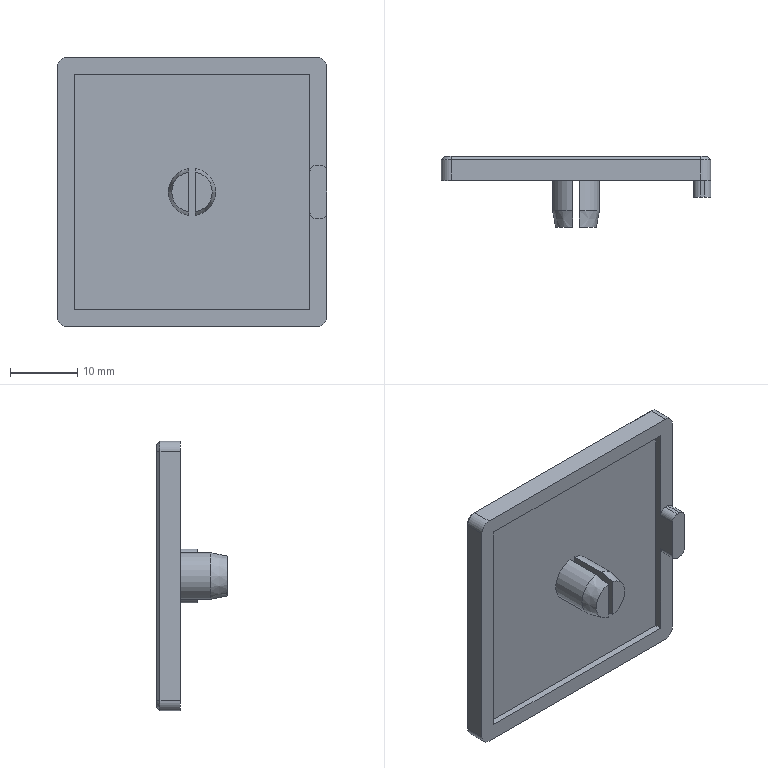Part | STEP file | 1 solid | 38 faces | box 40 x 10.5 x 40 mm | volume 4637 mm3 | plane 22 | cylinder 10 | cone 6 | commonest cylinder face diameters 2 x4 3 x4 7 x2